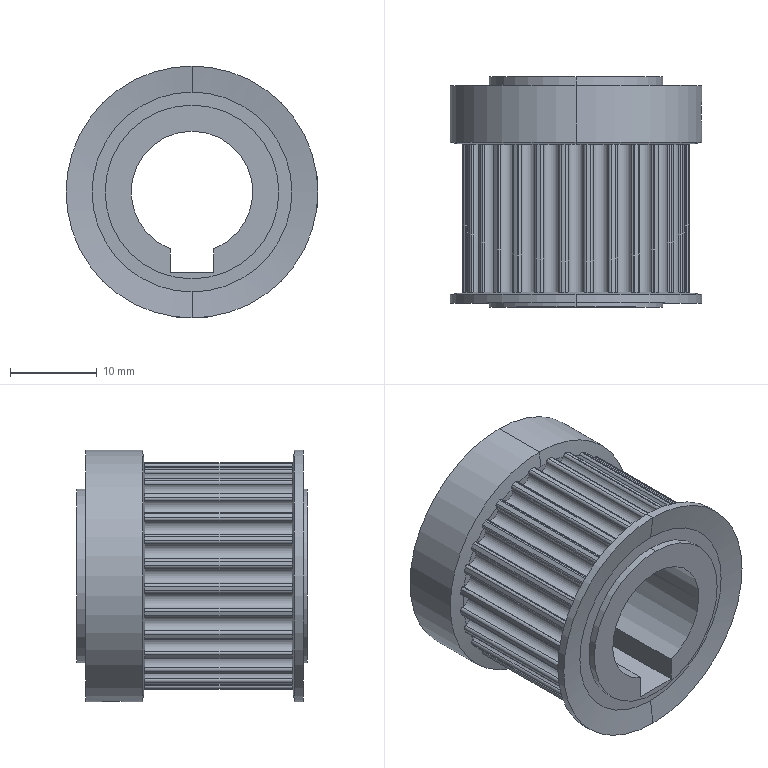Part | STEP file | 1 solid | 277 faces | box 29 x 26.5 x 29 mm | volume 9355 mm3 | cylinder 152 | plane 119 | cone 6 | commonest cylinder face diameters 0.665 x68 1.8 x42 26.22 x28 3.3 x4 20 x4 29 x4